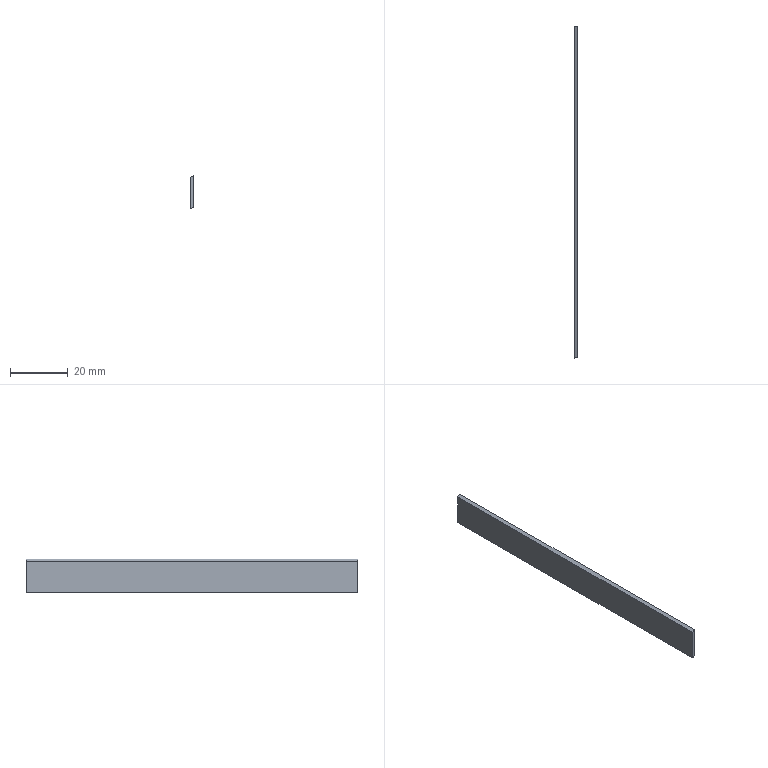Part | SolidWorks | features BaseBody 1 | 1 solid | 6 faces | box 1.056 x 115.104 x 11.504 mm | volume 1339 mm3 | plane 4 | cylinder 2 | commonest cylinder face diameters 97.2 x1 165.792 x1
STEP:
#1=CARTESIAN_POINT('',(-2108.29,1154.24,-1619.504));
#2=VERTEX_POINT('',#1);
#3=CARTESIAN_POINT('',(-2107.234,1154.24,-1618.864));
#4=VERTEX_POINT('',#3);
#5=CARTESIAN_POINT('',(-2132.95,1154.24,-1577.624));
#6=DIRECTION('',(0.,-1.,0.));
#7=DIRECTION('',(0.5074,0.,-0.8617));
#8=AXIS2_PLACEMENT_3D('',#5,#6,#7);
#9=CIRCLE('',#8,48.6);
#10=EDGE_CURVE('',#2,#4,#9,.T.);
#11=ORIENTED_EDGE('',*,*,#10,.T.);
#12=CARTESIAN_POINT('',(-2107.234,1269.344,-1618.864));
#13=VERTEX_POINT('',#12);
#14=CARTESIAN_POINT('',(-2107.234,1269.344,-1618.864));
#15=DIRECTION('',(0.,-1.,0.));
#16=VECTOR('',#15,1000.);
#17=LINE('',#14,#16);
#18=EDGE_CURVE('',#13,#4,#17,.T.);
#19=ORIENTED_EDGE('',*,*,#18,.F.);
#20=CARTESIAN_POINT('',(-2108.29,1269.344,-1619.504));
#21=VERTEX_POINT('',#20);
#22=CARTESIAN_POINT('',(-2132.95,1269.344,-1577.624));
#23=DIRECTION('',(0.,1.,0.));
#24=DIRECTION('',(0.5291,0.,-0.8485));
#25=AXIS2_PLACEMENT_3D('',#22,#23,#24);
#26=CIRCLE('',#25,48.6);
#27=EDGE_CURVE('',#13,#21,#26,.T.);
#28=ORIENTED_EDGE('',*,*,#27,.T.);
#29=CARTESIAN_POINT('',(-2108.29,1269.344,-1619.504));
#30=DIRECTION('',(0.,-1.,0.));
#31=VECTOR('',#30,1000.);
#32=LINE('',#29,#31);
#33=EDGE_CURVE('',#21,#2,#32,.T.);
#34=ORIENTED_EDGE('',*,*,#33,.T.);
#35=EDGE_LOOP('',(#11,#19,#28,#34));
#36=FACE_OUTER_BOUND('',#35,.T.);
#37=CARTESIAN_POINT('',(-2132.95,1275.099,-1577.624));
#38=DIRECTION('',(0.,-1.,0.));
#39=DIRECTION('',(0.4304,0.,-0.9027));
#40=AXIS2_PLACEMENT_3D('',#37,#38,#39);
#41=CYLINDRICAL_SURFACE('',#40,48.6);
#42=ADVANCED_FACE('',(#36),#41,.F.);
#43=CARTESIAN_POINT('',(-2107.234,1269.344,-1630.031));
#44=VERTEX_POINT('',#43);
#45=CARTESIAN_POINT('',(-2107.234,1154.24,-1630.031));
#46=VERTEX_POINT('',#45);
#47=CARTESIAN_POINT('',(-2107.234,1269.344,-1630.031));
#48=DIRECTION('',(0.,-1.,0.));
#49=VECTOR('',#48,1000.);
#50=LINE('',#47,#49);
#51=EDGE_CURVE('',#44,#46,#50,.T.);
#52=ORIENTED_EDGE('',*,*,#51,.T.);
#53=CARTESIAN_POINT('',(-2108.29,1154.24,-1630.368));
#54=VERTEX_POINT('',#53);
#55=CARTESIAN_POINT('',(-2132.95,1154.24,-1551.224));
#56=DIRECTION('',(0.,-1.,0.));
#57=DIRECTION('',(0.2975,0.,-0.9547));
#58=AXIS2_PLACEMENT_3D('',#55,#56,#57);
#59=CIRCLE('',#58,82.896);
#60=EDGE_CURVE('',#54,#46,#59,.T.);
#61=ORIENTED_EDGE('',*,*,#60,.F.);
#62=CARTESIAN_POINT('',(-2108.29,1269.344,-1630.368));
#63=VERTEX_POINT('',#62);
#64=CARTESIAN_POINT('',(-2108.29,1154.24,-1630.368));
#65=DIRECTION('',(0.,1.,0.));
#66=VECTOR('',#65,1000.);
#67=LINE('',#64,#66);
#68=EDGE_CURVE('',#54,#63,#67,.T.);
#69=ORIENTED_EDGE('',*,*,#68,.T.);
#70=CARTESIAN_POINT('',(-2132.95,1269.344,-1551.224));
#71=DIRECTION('',(0.,1.,0.));
#72=DIRECTION('',(0.3102,0.,-0.9507));
#73=AXIS2_PLACEMENT_3D('',#70,#71,#72);
#74=CIRCLE('',#73,82.896);
#75=EDGE_CURVE('',#44,#63,#74,.T.);
#76=ORIENTED_EDGE('',*,*,#75,.F.);
#77=EDGE_LOOP('',(#52,#61,#69,#76));
#78=FACE_OUTER_BOUND('',#77,.T.);
#79=CARTESIAN_POINT('',(-2132.95,1275.099,-1551.224));
#80=DIRECTION('',(0.,1.,0.));
#81=DIRECTION('',(0.3919,0.,-0.92));
#82=AXIS2_PLACEMENT_3D('',#79,#80,#81);
#83=CYLINDRICAL_SURFACE('',#82,82.896);
#84=ADVANCED_FACE('',(#78),#83,.T.);
#85=ORIENTED_EDGE('',*,*,#27,.F.);
#86=CARTESIAN_POINT('',(-2107.234,1269.344,-1618.864));
#87=DIRECTION('',(0.000000008,-0.000000002,-1.));
#88=VECTOR('',#87,1000.);
#89=LINE('',#86,#88);
#90=EDGE_CURVE('',#13,#44,#89,.T.);
#91=ORIENTED_EDGE('',*,*,#90,.T.);
#92=ORIENTED_EDGE('',*,*,#75,.T.);
#93=CARTESIAN_POINT('',(-2108.29,1269.344,-1630.368));
#94=DIRECTION('',(0.000000009,0.000000002,1.));
#95=VECTOR('',#94,1000.);
#96=LINE('',#93,#95);
#97=EDGE_CURVE('',#63,#21,#96,.T.);
#98=ORIENTED_EDGE('',*,*,#97,.T.);
#99=EDGE_LOOP('',(#85,#91,#92,#98));
#100=FACE_OUTER_BOUND('',#99,.T.);
#101=CARTESIAN_POINT('',(-2106.659,1269.344,-1630.943));
#102=DIRECTION('',(0.,1.,0.));
#103=DIRECTION('',(1.,0.,0.));
#104=AXIS2_PLACEMENT_3D('',#101,#102,#103);
#105=PLANE('',#104);
#106=ADVANCED_FACE('',(#100),#105,.T.);
#107=ORIENTED_EDGE('',*,*,#10,.F.);
#108=CARTESIAN_POINT('',(-2108.29,1154.24,-1619.504));
#109=DIRECTION('',(-0.000000005,0.000000002,-1.));
#110=VECTOR('',#109,1000.);
#111=LINE('',#108,#110);
#112=EDGE_CURVE('',#2,#54,#111,.T.);
#113=ORIENTED_EDGE('',*,*,#112,.T.);
#114=ORIENTED_EDGE('',*,*,#60,.T.);
#115=CARTESIAN_POINT('',(-2107.234,1154.24,-1630.031));
#116=DIRECTION('',(-0.000000008,-0.000000002,1.));
#117=VECTOR('',#116,1000.);
#118=LINE('',#115,#117);
#119=EDGE_CURVE('',#46,#4,#118,.T.);
#120=ORIENTED_EDGE('',*,*,#119,.T.);
#121=EDGE_LOOP('',(#107,#113,#114,#120));
#122=FACE_OUTER_BOUND('',#121,.T.);
#123=CARTESIAN_POINT('',(-2108.865,1154.24,-1630.943));
#124=DIRECTION('',(0.,-1.,0.));
#125=DIRECTION('',(0.,0.,-1.));
#126=AXIS2_PLACEMENT_3D('',#123,#124,#125);
#127=PLANE('',#126);
#128=ADVANCED_FACE('',(#122),#127,.T.);
#129=ORIENTED_EDGE('',*,*,#68,.F.);
#130=ORIENTED_EDGE('',*,*,#112,.F.);
#131=ORIENTED_EDGE('',*,*,#33,.F.);
#132=ORIENTED_EDGE('',*,*,#97,.F.);
#133=EDGE_LOOP('',(#129,#130,#131,#132));
#134=FACE_OUTER_BOUND('',#133,.T.);
#135=CARTESIAN_POINT('',(-2108.29,1275.099,-1613.748));
#136=DIRECTION('',(-1.,0.,0.));
#137=DIRECTION('',(0.,0.,1.));
#138=AXIS2_PLACEMENT_3D('',#135,#136,#137);
#139=PLANE('',#138);
#140=ADVANCED_FACE('',(#134),#139,.T.);
#141=ORIENTED_EDGE('',*,*,#18,.T.);
#142=ORIENTED_EDGE('',*,*,#119,.F.);
#143=ORIENTED_EDGE('',*,*,#51,.F.);
#144=ORIENTED_EDGE('',*,*,#90,.F.);
#145=EDGE_LOOP('',(#141,#142,#143,#144));
#146=FACE_OUTER_BOUND('',#145,.T.);
#147=CARTESIAN_POINT('',(-2107.234,1275.099,-1635.786));
#148=DIRECTION('',(1.,0.,0.));
#149=DIRECTION('',(0.,1.,0.));
#150=AXIS2_PLACEMENT_3D('',#147,#148,#149);
#151=PLANE('',#150);
#152=ADVANCED_FACE('',(#146),#151,.T.);
#153=CLOSED_SHELL('',(#42,#84,#106,#128,#140,#152));
#154=MANIFOLD_SOLID_BREP('',#153);
#155=CARTESIAN_POINT('',(0.,0.,0.));
#156=DIRECTION('',(0.,0.,1.));
#157=DIRECTION('',(1.,0.,0.));
#158=AXIS2_PLACEMENT_3D('',#155,#156,#157);
#159=(LENGTH_UNIT()NAMED_UNIT(*)SI_UNIT(.MILLI.,.METRE.));
#160=UNCERTAINTY_MEASURE_WITH_UNIT(LENGTH_MEASURE(0.00001),#159,'','');
#161=(NAMED_UNIT(*)PLANE_ANGLE_UNIT()SI_UNIT($,.RADIAN.));
#162=(NAMED_UNIT(*)SI_UNIT($,.STERADIAN.)SOLID_ANGLE_UNIT());
#163=(GEOMETRIC_REPRESENTATION_CONTEXT(3)GLOBAL_UNCERTAINTY_ASSIGNED_CONTEXT((#160))GLOBAL_UNIT_ASSIGNED_CONTEXT((#159,#161,#162))REPRESENTATION_CONTEXT('',''));
#164=ADVANCED_BREP_SHAPE_REPRESENTATION('',(#154,#158),#163);